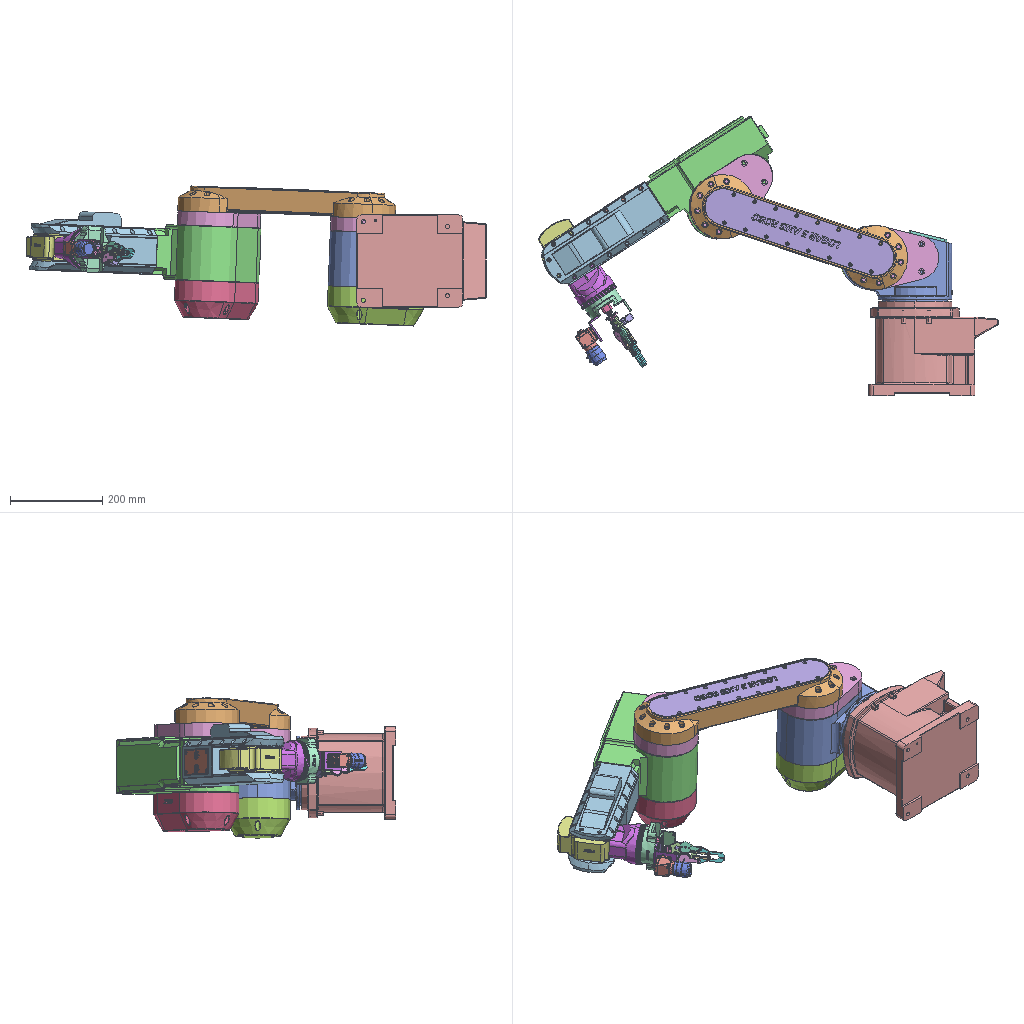Assembly | SolidWorks | 49 different items | 76 placed | box 997 x 606 x 304 mm
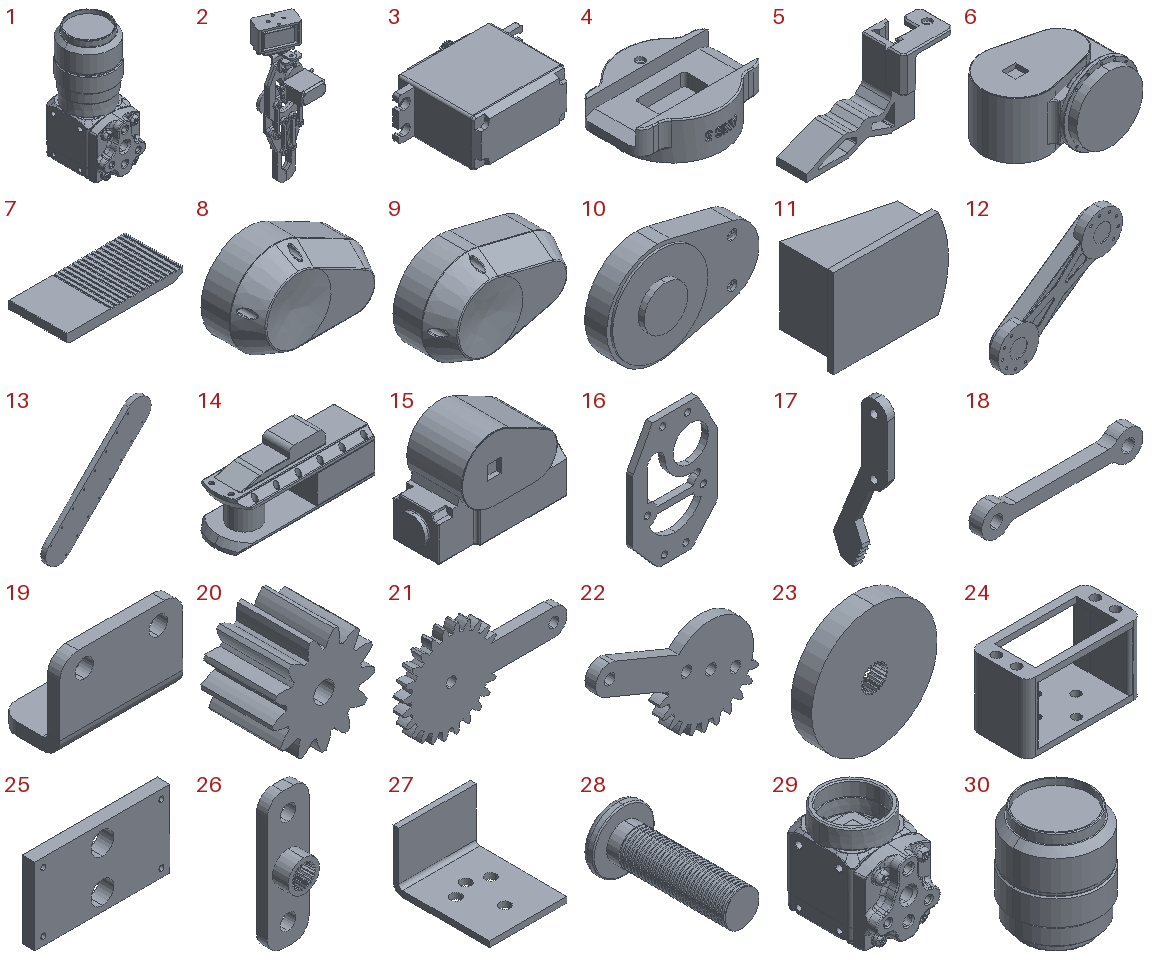Parts list (item | name | quantity | parent item | size | volume | features):
1 | (subassembly) | x1 | - | - | - | -
2 | (subassembly) | x1 | - | 55.908 x 54.775 x 166.65 mm | 52779 mm3 | features CompositeCurve 4, AEMSimFeature 1
3 | (subassembly) | x1 | in 2 | 38.29 x 31.325 x 14.35 mm | 10527 mm3 | -
4 | - | x1 | - | 100 x 81 x 40 mm | 134637 mm3 | features ICE 4, Fillet 3, 3DProfileFeature 1, Chamfer 1, Emboss 1, Extrusion 1, HoleWzd 1
5 | - | x1 | - | 107 x 39 x 65 mm | 37436 mm3 | features ICE 7, Chamfer 6, Fillet 2, 3DProfileFeature 1, Extrusion 1, HoleWzd 1
6 | - | x1 | - | 241 x 179 x 160 mm | 3546653 mm3 | features ICE 11, CirPattern 3, Fillet 3, MirrorPattern 2, 3DProfileFeature 1, Chamfer 1, Emboss 1, Extrusion 1, HoleWzd 1
7 | - | x1 | - | 50 x 25 x 9.5 mm | 5299 mm3 | features Chamfer 2, ICE 2, Extrusion 1, LPattern 1
8 | - | x1 | - | 208 x 90 x 141 mm | 1602539 mm3 | features ICE 3, CirPattern 2, Fillet 2, Chamfer 1, Dome 1, Emboss 1, Extrusion 1, PLine 1
9 | - | x1 | - | 208.413 x 90 x 140 mm | 1586801 mm3 | features ICE 5, Fillet 2, Chamfer 1, CirPattern 1, Dome 1, Extrusion 1, PLine 1
10 | - | x2 | - | 208.413 x 51.01 x 140 mm | 738708 mm3 | features ICE 3, 3DProfileFeature 1, Extrusion 1, HoleWzd 1
11 | - | x1 | - | 90.603 x 47.87 x 70 mm | 179033 mm3 | features ICE 4, Extrusion 1, Fillet 1
12 | - | x1 | - | 426.703 x 55 x 340.752 mm | 1944571 mm3 | features ICE 6, Fillet 5, Chamfer 1, CirPattern 1, Emboss 1, Extrusion 1, MirrorPattern 1
13 | - | x1 | - | 327.487 x 16 x 327.487 mm | 460753 mm3 | features ICE 3, Emboss 1, Extrusion 1, LPattern 1, MirrorPattern 1
14 | - | x1 | - | 280 x 100 x 130 mm | 1901743 mm3 | features ICE 13, Fillet 4, Chamfer 3, LPattern 2, 3DProfileFeature 1, Extrusion 1, HoleWzd 1
15 | - | x1 | - | 290 x 120 x 210 mm | 5097544 mm3 | features ICE 7, Chamfer 4, MirrorPattern 2, Extrusion 1, Fillet 1
16 | - | x2 | in 2 | 40.999 x 3 x 62 mm | 4212 mm3 | features Extrusion 1, Fillet 1
17 | - | x4 | in 2 | 3 x 20.791 x 60.365 mm | 1428 mm3 | features ICE 3, Extrusion 1
18 | - | x6 | in 2 | 38 x 3 x 7 mm | 409.975 mm3 | features Extrusion 1, Fillet 1
19 | - | x2 | in 2 | 20 x 10 x 14 mm | 792.323 mm3 | features ICE 2, Fillet 1, FlatPattern 1, SMBaseFlange 1, SheetMetal 1
20 | - | x1 | in 2 | 14.953 x 10.5 x 14.85 mm | 1337 mm3 | features Extrusion 1, ICE 1
21 | - | x1 | in 2 | 49.537 x 3 x 29.075 mm | 2135 mm3 | features Extrusion 1
22 | - | x1 | in 2 | 46.268 x 3 x 30.401 mm | 1962 mm3 | features ICE 2, Extrusion 1
23 | - | x1 | in 2 | 21 x 3.5 x 21 mm | 1045 mm3 | features CombineBodies 1, Extrusion 1, ICE 1, MoveCopyBody 1, Stock 1
24 | - | x1 | in 2 | 40 x 20 x 24 mm | 5034 mm3 | features ICE 5, Fillet 2, Extrusion 1
25 | - | x1 | - | 95 x 10.05 x 54 mm | 46492 mm3 | features ICE 2, 3DProfileFeature 1, Chamfer 1, Extrusion 1, HoleWzd 1
26 | - | x1 | in 2 | 8 x 5 x 26 mm | 406.224 mm3 | features ICE 2, CombineBodies 1, Extrusion 1, MoveCopyBody 1, Stock 1
27 | - | x1 | - | 40 x 50 x 30 mm | 8775 mm3 | features EdgeFlange 1, FlatPattern 1, HoleWzd 1, SMBaseFlange 1, SheetMetal 1
28 | - | x1 | - | 5.3 x 11.1 x 5.3 mm | 89.179 mm3 | features Fillet 2, Helix 2, ICE 2, SweepCut 2, Extrusion 1
29 | - | x1 | in 1 | - | - | features RefSurface 1
30 | - | x1 | in 1 | - | - | features RefSurface 1
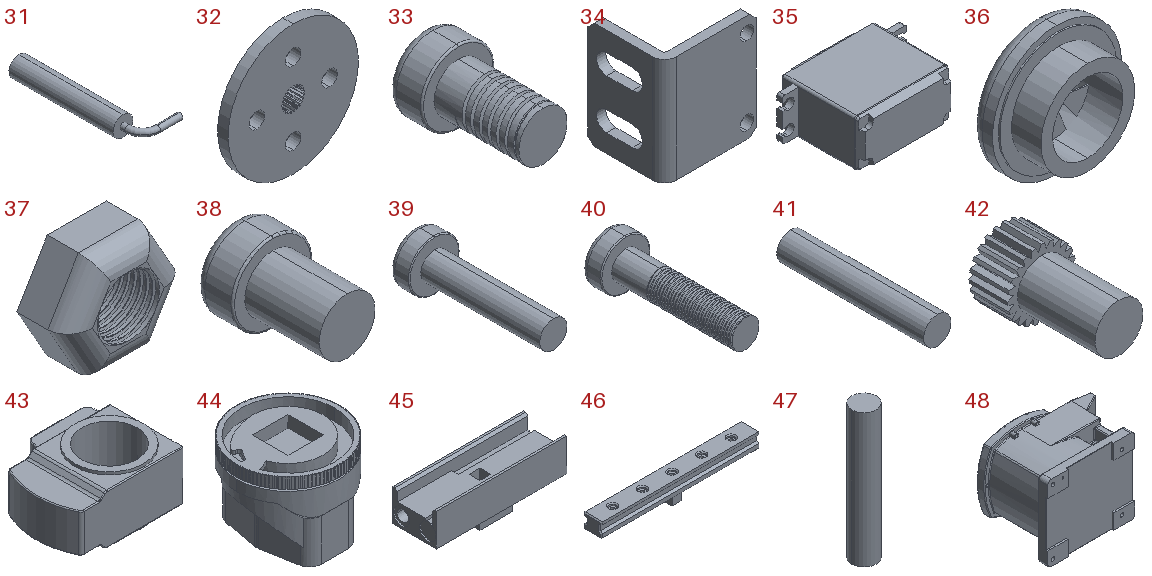31 | - | x1 | - | 19 x 51.25 x 8 mm | 2211 mm3 | features Extrusion 1, PLine 1, Sweep 1
32 | - | x1 | - | 25 x 4.2 x 25 mm | 966.612 mm3 | features ICE 5, CirPattern 1, CombineBodies 1, Extrusion 1, MoveCopyBody 1, Stock 1
33 | - | x1 | - | 4.3 x 7 x 4.3 mm | 56.462 mm3 | features Helix 3, SweepCut 3, Fillet 2, ICE 2, Extrusion 1
34 | - | x1 | - | 30 x 25 x 35 mm | 4690 mm3 | features ICE 3, Chamfer 2, DelFace 2, HoleWzd 2, MoveFace 2, BaseBody 1
35 | - | x2 | in 2, 3 | 38.29 x 27.125 x 14.35 mm | 10479 mm3 | features ICE 14, RevCut 4, Fillet 2, Rib 2, Chamfer 1, Extrusion 1, Revolution 1, Scale 1
36 | - | x2 | - | 22 x 9 x 22 mm | 1452 mm3 | features ICE 4, Extrusion 1, Fillet 1
37 | - | x2 | in 2 | 5.773 x 2.5 x 5.023 mm | 33.605 mm3 | features CombineBodies 1, Extrusion 1, Fillet 1, ICE 1, MoveCopyBody 1, Stock 1
38 | - | x5 | in 2 | 4.3 x 6 x 4.3 mm | 53.843 mm3 | features Fillet 2, ICE 2, Extrusion 1
39 | - | x1 | in 2 | 5.3 x 14.5 x 5.3 mm | 122.133 mm3 | features Fillet 2, ICE 2, Extrusion 1, Helix 1
40 | - | x2 | in 2 | 5.3 x 14.8 x 5.3 mm | 130.333 mm3 | features Fillet 2, Helix 2, ICE 2, SweepCut 2, Extrusion 1
41 | - | x8 | in 2 | 3 x 16 x 3 mm | 113.097 mm3 | features Extrusion 1
42 | - | x2 | in 2, 3 | 4.357 x 7.5 x 4.358 mm | 48.395 mm3 | features CombineBodies 2, MoveCopyBody 2, Stock 2, Extrusion 1, ICE 1
43 | - | x1 | - | 132 x 97 x 60 mm | 392584 mm3 | features ICE 6, Fillet 3, Emboss 1, Extrusion 1, MirrorPattern 1
44 | - | x1 | - | 88 x 88 x 70 mm | 300760 mm3 | features ICE 7, Chamfer 3, Fillet 2, CirPattern 1, Extrusion 1, RevCut 1
45 | - | x1 | - | 120 x 40 x 40 mm | 99907 mm3 | features ICE 7, Chamfer 1, Extrusion 1, MirrorPattern 1
46 | - | x1 | - | 160 x 18 x 25 mm | 37654 mm3 | features Chamfer 3, ICE 2, 3DProfileFeature 1, Extrusion 1, HoleWzd 1, LPattern 1, MirrorPattern 1
47 | - | x1 | - | 10 x 10 x 55 mm | 4320 mm3 | features Extrusion 1
48 | - | x1 | - | 280 x 205 x 200 mm | 6648707 mm3 | features ICE 12, Fillet 7, 3DProfileFeature 2, Chamfer 2, HoleWzd 2, MirrorPattern 2, Extrusion 1
49 | Small TypePhotoelectric-Optex CX-441 | x1 | - | - | - | -
Mates (type | each side: item.copy, entity, surface, feature):
In the top assembly
Coincident | 48.1 edge | 6.1 edge
LimitPlanarAngleDim | 48.1 plane | 6.1 plane
Concentric | 6.1 edge | 9.1 edge
Coincident | 6.1 face plane Mirror1 | 9.1 face plane Boss-Extrude1
Parallel | 6.1 face plane Boss-Extrude3 | 9.1 face plane Boss-Extrude1
Parallel | 6.1 face plane Boss-Extrude3 | 10.1 face plane Boss-Extrude1
Concentric | 6.1 edge | 10.1 edge
Coincident | 6.1 face plane Boss-Extrude4 | 10.1 face plane Boss-Extrude1
Parallel | 6.1 face plane Boss-Extrude3 | 11.1 face plane Cut-Extrude1
Coincident | 6.1 edge | 11.1 edge
Coincident | 6.1 face plane Cut-Extrude1 | 11.1 face plane Boss-Extrude1
Coincident | 10.1 edge | 12.1 edge
LimitPlanarAngleDim | 12.1 plane | 6.1 plane
Coincident | 12.1 face plane Cut-Extrude2 | 13.1 face plane Boss-Extrude1
Concentric | 12.1 face cylinder Cut-Extrude2 | 13.1 face cylinder Boss-Extrude1
Concentric | 12.1 edge | 13.1 edge
Coincident | 12.1 edge | 10.2 edge
LimitPlanarAngleDim | 10.2 plane | 12.1 plane
Coincident | 10.2 face plane Boss-Extrude1 | 15.1 face plane Boss-Extrude1
Concentric | 12.1 face cylinder Boss-Extrude1 | 15.1 face cylinder Boss-Extrude1
Parallel | 10.2 face plane Boss-Extrude1 | 15.1 face plane Boss-Extrude2
Coincident | 15.1 face plane Boss-Extrude1 | 8.1 face plane Boss-Extrude1
Concentric | 15.1 face cylinder Boss-Extrude1 | 8.1 face cylinder Boss-Extrude1
Parallel | 15.1 face plane Boss-Extrude2 | 8.1 face plane Boss-Extrude1
Concentric | 15.1 edge | 14.1 edge
Coincident | 15.1 face plane Boss-Extrude2 | 14.1 face plane Boss-Extrude1
Parallel | 15.1 face plane Boss-Extrude2 | 14.1 face plane Cut-Extrude5
Concentric | 14.1 face cylinder Boss-Extrude2 | 43.1 face cylinder Cut-Extrude1
Coincident | 14.1 plane | 43.1 plane
LimitPlanarAngleDim | 14.1 plane | 43.1 plane
Coincident | 43.1 face plane Boss-Extrude4 | 44.1 face plane Cut-Extrude1 | 2 times
Coincident | 43.1 face plane Boss-Extrude1 | 44.1 face plane Boss-Extrude1
Concentric | 44.1 face cylinder Cut-Extrude2 | 4.1 face cylinder Boss-Extrude1
Coincident | 44.1 face plane Cut-Extrude3 | 4.1 face plane Boss-Extrude2 | 2 times
Coincident | 14.1 face plane Cut-Extrude5 | 25.1 face plane Boss-Extrude1 | 2 times
Coincident | 14.1 face plane Cut-Extrude5 | 25.1 edge
Concentric | 25.1 face cylinder Cut-Extrude2 | 36.1 face cylinder Boss-Extrude1
Coincident | 14.1 face plane Cut-Extrude5 | 36.1 edge
Concentric | 25.1 face cylinder Cut-Extrude2 | 36.2 face cylinder Boss-Extrude1
Coincident | 14.1 face plane Cut-Extrude5 | 36.2 edge
Coincident | 4.1 face plane Cut-Extrude1 | 24.1 face plane Boss-Extrude3
Coincident | 4.1 face plane Cut-Extrude1 | 24.1 face plane Boss-Extrude1 | 2 times
Coincident | 4.1 face plane Boss-Extrude4 | 27.1 face plane Edge-Flange1 | 2 times
Parallel | 24.1 face plane Boss-Extrude1 | 27.1 face plane Edge-Flange1
Width | 4.1 face plane Boss-Extrude3 | 4.1 face plane Boss-Extrude3 | 27.1 face plane Edge-Flange1 | 27.1 face plane Edge-Flange1
Coincident | 27.1 face plane Base-Flange1 | 29.1 face plane Surface-input1
DistanceDim | 29.1 face plane Surface-input1 | 27.1 face plane Base-Flange1
Width | 29.1 face plane Surface-input1 | 29.1 face plane Surface-input1 | 27.1 face plane Base-Flange1 | 27.1 face plane Base-Flange1
Coincident | 4.1 face plane Boss-Extrude4 | 34.1 face plane Boss-Extrude1
DistanceDim | 34.1 face plane Input1 | 4.1 face plane Boss-Extrude4
Coincident | 27.1 face plane Edge-Flange1 | 34.1 face plane Input1
In subassembly 2
Coincident | 16.1 face plane Boss-Extrude1 | 16.2 face plane Boss-Extrude1
Concentric | 16.1 face cylinder Boss-Extrude1 | 16.2 face cylinder Boss-Extrude1 | 2 times
Coincident | 16.1 face plane Boss-Extrude1 | 19.1 face plane Base-Flange1
Concentric | 16.2 face cylinder Boss-Extrude1 | 19.1 face cylinder Cut-Extrude1
Coincident | 16.2 face plane Boss-Extrude1 | 19.2 face plane Base-Flange1
Concentric | 16.2 face cylinder Boss-Extrude1 | 19.2 face cylinder Cut-Extrude1 | 2 times
Coincident | 17.1 face plane Boss-Extrude1 | 17.2 face plane Boss-Extrude1
Concentric | 17.1 face cylinder Boss-Extrude1 | 17.2 face cylinder Boss-Extrude1 | 2 times
Coincident | 17.3 face plane Boss-Extrude1 | 17.4 face plane Boss-Extrude1
Concentric | 17.3 face cylinder Boss-Extrude1 | 17.4 face cylinder Boss-Extrude1 | 2 times
DistanceDim | 16.1 face plane Boss-Extrude1 | 18.1 face plane Boss-Extrude1
Concentric | 16.1 face cylinder Boss-Extrude1 | 18.1 face cylinder Boss-Extrude1
Concentric | 17.2 face cylinder Boss-Extrude1 | 18.1 face cylinder Boss-Extrude1
DistanceDim | 18.2 face plane Boss-Extrude1 | 16.1 face plane Boss-Extrude1
Concentric | 16.1 face cylinder Boss-Extrude1 | 18.2 face cylinder Boss-Extrude1
Concentric | 17.4 face cylinder Boss-Extrude1 | 18.2 face cylinder Boss-Extrude1
DistanceDim | 18.3 face plane Boss-Extrude1 | 16.1 face plane Boss-Extrude1
Concentric | 16.1 face cylinder Boss-Extrude1 | 18.3 face cylinder Boss-Extrude1
Concentric | 17.4 face cylinder Boss-Extrude1 | 18.3 face cylinder Boss-Extrude1
DistanceDim | 18.4 face plane Boss-Extrude1 | 16.2 face plane Boss-Extrude1
Concentric | 16.2 face cylinder Boss-Extrude1 | 18.4 face cylinder Boss-Extrude1
Concentric | 17.3 face cylinder Boss-Extrude1 | 18.4 face cylinder Boss-Extrude1
DistanceDim | 16.1 face plane Boss-Extrude1 | 18.5 face plane Boss-Extrude1
Concentric | 16.1 face cylinder Boss-Extrude1 | 18.5 face cylinder Boss-Extrude1
Concentric | 17.2 face cylinder Boss-Extrude1 | 18.5 face cylinder Boss-Extrude1
DistanceDim | 18.6 face plane Boss-Extrude1 | 16.2 face plane Boss-Extrude1
Concentric | 16.2 face cylinder Boss-Extrude1 | 18.6 face cylinder Boss-Extrude1
Concentric | 17.1 face cylinder Boss-Extrude1 | 18.6 face cylinder Boss-Extrude1
DistanceDim | 17.4 face plane Boss-Extrude1 | 18.2 face plane Boss-Extrude1
DistanceDim | 18.1 face plane Boss-Extrude1 | 17.2 face plane Boss-Extrude1
Concentric | 16.2 face cylinder Boss-Extrude1 | 20.1 face cylinder Cut-Extrude1
Concentric | 16.1 face cylinder Boss-Extrude1 | 19.1 face cylinder Cut-Extrude1
Concentric | 20.1 face cylinder Cut-Extrude1 | 23.1 face cylinder Boss-Extrude1
Coincident | 20.1 face plane Boss-Extrude1 | 23.1 face plane Cut-Extrude1
Concentric | 20.1 face cylinder Cut-Extrude1 | 39.1 face cylinder Boss-Extrude2
Coincident | 20.1 face plane Boss-Extrude1 | 39.1 face plane Boss-Extrude1
Concentric | 19.2 face cylinder Cut-Extrude1 | 40.1 face cylinder Boss-Extrude2
Coincident | 19.2 face plane Base-Flange1 | 40.1 face plane Boss-Extrude1
Concentric | 19.2 face cylinder Cut-Extrude1 | 40.2 face cylinder Boss-Extrude2
Coincident | 19.2 face plane Base-Flange1 | 40.2 face plane Boss-Extrude1
Concentric | 40.1 face cylinder Boss-Extrude2 | 37.1 face cylinder Combine1
Coincident | 19.1 face plane Base-Flange1 | 37.1 face plane Boss-Extrude1
Concentric | 40.2 face cylinder Boss-Extrude2 | 37.2 face cylinder Combine1
Coincident | 19.1 face plane Base-Flange1 | 37.2 face plane Boss-Extrude1
Tangent | 20.1 face cylinder Boss-Extrude1 | 23.1 face cylinder Cut-Extrude1
Concentric | 17.1 face cylinder Boss-Extrude1 | 21.1 face cylinder Boss-Extrude1
Concentric | 16.2 face cylinder Boss-Extrude1 | 21.1 face cylinder Boss-Extrude1
DistanceDim | 21.1 face plane Boss-Extrude1 | 16.2 face plane Boss-Extrude1
Concentric | 16.2 face cylinder Boss-Extrude1 | 22.1 face cylinder Boss-Extrude1
Concentric | 17.3 face cylinder Boss-Extrude1 | 22.1 face cylinder Boss-Extrude2
DistanceDim | 22.1 face plane Boss-Extrude1 | 16.2 face plane Boss-Extrude1
GearDim | 22.1 edge | 21.1 edge
Coincident | 16.1 face plane Boss-Extrude1 | 41.1 plane
Concentric | 21.1 face cylinder Boss-Extrude1 | 41.1 face cylinder Boss-Extrude1
Concentric | 21.1 face cylinder Boss-Extrude1 | 41.2 face cylinder Boss-Extrude1
Coincident | 41.1 face plane Boss-Extrude1 | 41.2 face plane Boss-Extrude1
Concentric | 22.1 face cylinder Boss-Extrude1 | 41.3 face cylinder Boss-Extrude1
Coincident | 41.1 face plane Boss-Extrude1 | 41.3 face plane Boss-Extrude1
Concentric | 18.6 face cylinder Boss-Extrude1 | 41.4 face cylinder Boss-Extrude1
Coincident | 41.1 face plane Boss-Extrude1 | 41.4 face plane Boss-Extrude1
Coincident | 41.3 face plane Boss-Extrude1 | 41.5 face plane Boss-Extrude1
Concentric | 22.1 face cylinder Boss-Extrude2 | 41.5 face cylinder Boss-Extrude1
Coincident | 41.4 face plane Boss-Extrude1 | 41.6 face plane Boss-Extrude1
Concentric | 18.6 face cylinder Boss-Extrude1 | 41.6 face cylinder Boss-Extrude1
Coincident | 41.6 face plane Boss-Extrude1 | 41.7 face plane Boss-Extrude1
Concentric | 18.4 face cylinder Boss-Extrude1 | 41.7 face cylinder Boss-Extrude1
Coincident | 41.4 face plane Boss-Extrude1 | 41.8 face plane Boss-Extrude1
Concentric | 18.4 face cylinder Boss-Extrude1 | 41.8 face cylinder Boss-Extrude1
GearDim | 20.1 edge | 21.1 edge
Concentric | 23.1 face cylinder Boss-Extrude1 | 42.1 face cylinder Boss-Extrude1
Coincident | 23.1 face plane Combine1 | 42.1 face plane Combine1
Coincident | 23.1 face plane Cut-Extrude1 | 42.1 face plane Boss-Extrude2
DistanceDim | 21.1 face plane Boss-Extrude1 | 20.1 face plane Boss-Extrude1
Parallel | 16.1 face plane Boss-Extrude1 | 35.1 face plane Boss-Extrude2
LimitPlanarAngleDim | 22.1 face plane Boss-Extrude2 | 16.2 face plane Boss-Extrude1
Coincident | 35.2 face plane Boss-Extrude3 | 24.2 face plane Boss-Extrude1
Parallel | 35.2 face plane Boss-Extrude2 | 24.2 face plane Boss-Extrude2
Tangent | 35.2 face cylinder Cut-Revolve4 | 24.2 face cylinder Cut-Extrude2
Concentric | 35.2 face cylinder Cut-Revolve4 | 24.2 face cylinder Cut-Extrude2
Concentric | 35.2 face cylinder Cut-Revolve3 | 24.2 face cylinder Cut-Extrude2
Concentric | 35.2 face cylinder Cut-Revolve1 | 24.2 face cylinder Cut-Extrude2
Concentric | 35.2 face cylinder Cut-Extrude10 | 42.2 face cylinder Boss-Extrude1
Coincident | 35.2 face plane Revolve1 | 42.2 face plane Boss-Extrude2
Coincident | 26.1 face plane Combine1 | 42.2 face plane Boss-Extrude2
Concentric | 26.1 face cylinder Boss-Extrude2 | 42.2 face cylinder Combine3
Parallel | 19.2 face plane Base-Flange1 | 35.2 face plane Boss-Extrude5
Coincident | 19.2 face plane Base-Flange1 | 26.1 face plane Boss-Extrude1
Concentric | 19.2 face cylinder Cut-Extrude2 | 26.1 face cylinder Boss-Extrude1
Concentric | 19.1 face cylinder Cut-Extrude2 | 26.1 face cylinder Boss-Extrude1
Concentric | 35.2 face cylinder Cut-Revolve3 | 38.1 face cylinder Boss-Extrude2
Coincident | 35.2 face plane Boss-Extrude3 | 38.1 face plane Boss-Extrude1
Concentric | 35.2 face cylinder Cut-Revolve4 | 38.2 face cylinder Boss-Extrude2
Coincident | 35.2 face plane Boss-Extrude3 | 38.2 face plane Boss-Extrude1
Concentric | 35.2 face cylinder Cut-Revolve2 | 38.3 face cylinder Boss-Extrude2
Coincident | 35.2 face plane Boss-Extrude4 | 38.3 face plane Boss-Extrude1
Concentric | 35.2 face cylinder Cut-Revolve1 | 38.4 face cylinder Boss-Extrude2
Coincident | 35.2 face plane Boss-Extrude4 | 38.4 face plane Boss-Extrude1
Concentric | 19.2 face cylinder Cut-Extrude2 | 38.5 face cylinder Boss-Extrude2
Coincident | 19.2 face plane Base-Flange1 | 38.5 face plane Boss-Extrude1
In subassembly 3
Concentric | 35.2 face cylinder Cut-Extrude10 | 42.2 face cylinder Boss-Extrude1
DistanceDim | 42.2 face plane Boss-Extrude2 | 35.2 face plane Revolve1